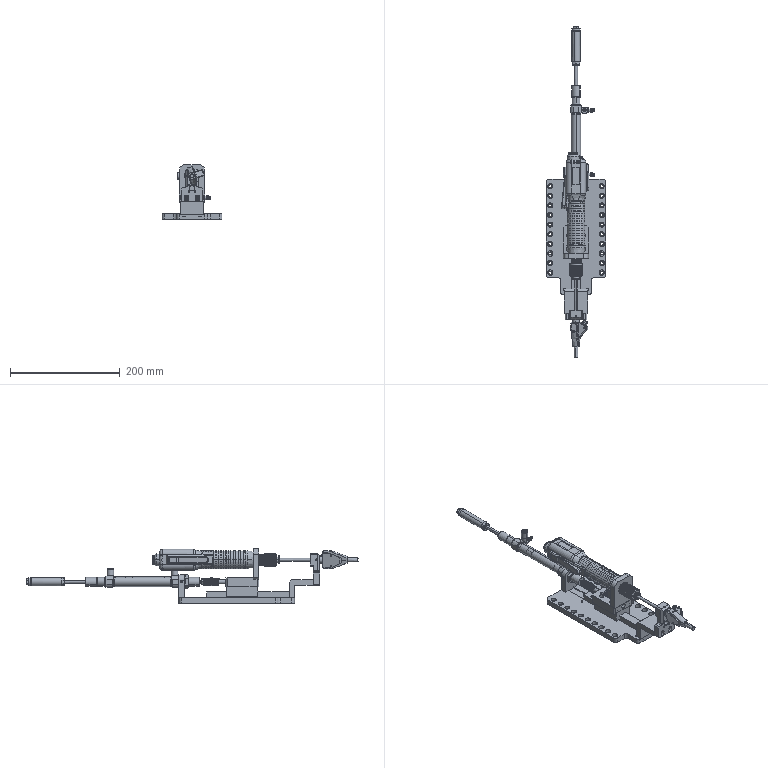Part | SolidWorks | 25 solids | 2698 faces | box 108.9 x 604.66 x 99 mm | volume 644480 mm3 | cylinder 1304 | plane 698 | spline 403 | cone 163 | torus 123 | sphere 7 | commonest cylinder face diameters 0.494 x150 0.716 x140 4.724 x56 5.2 x56 6.564 x56 7.04 x56